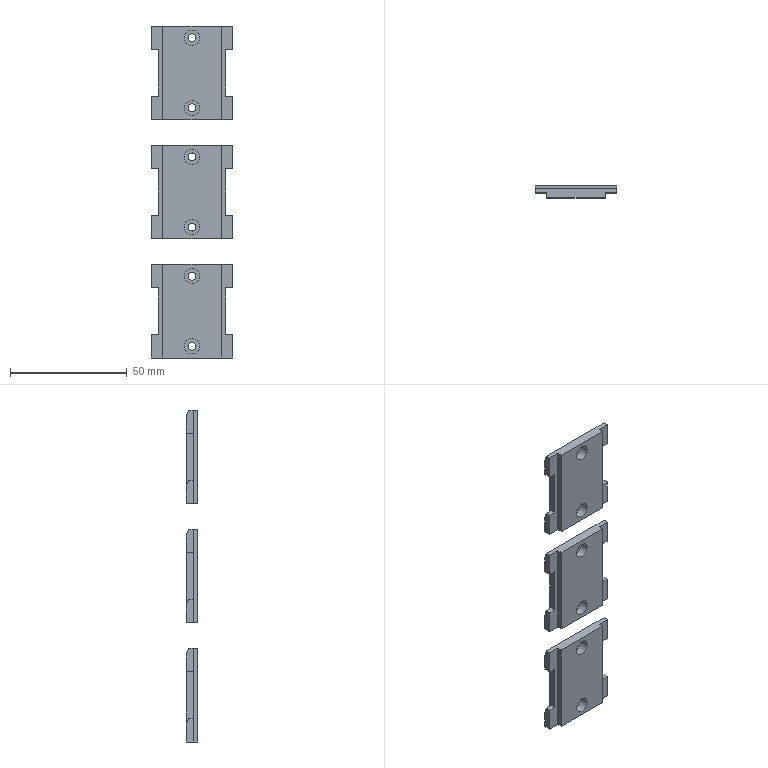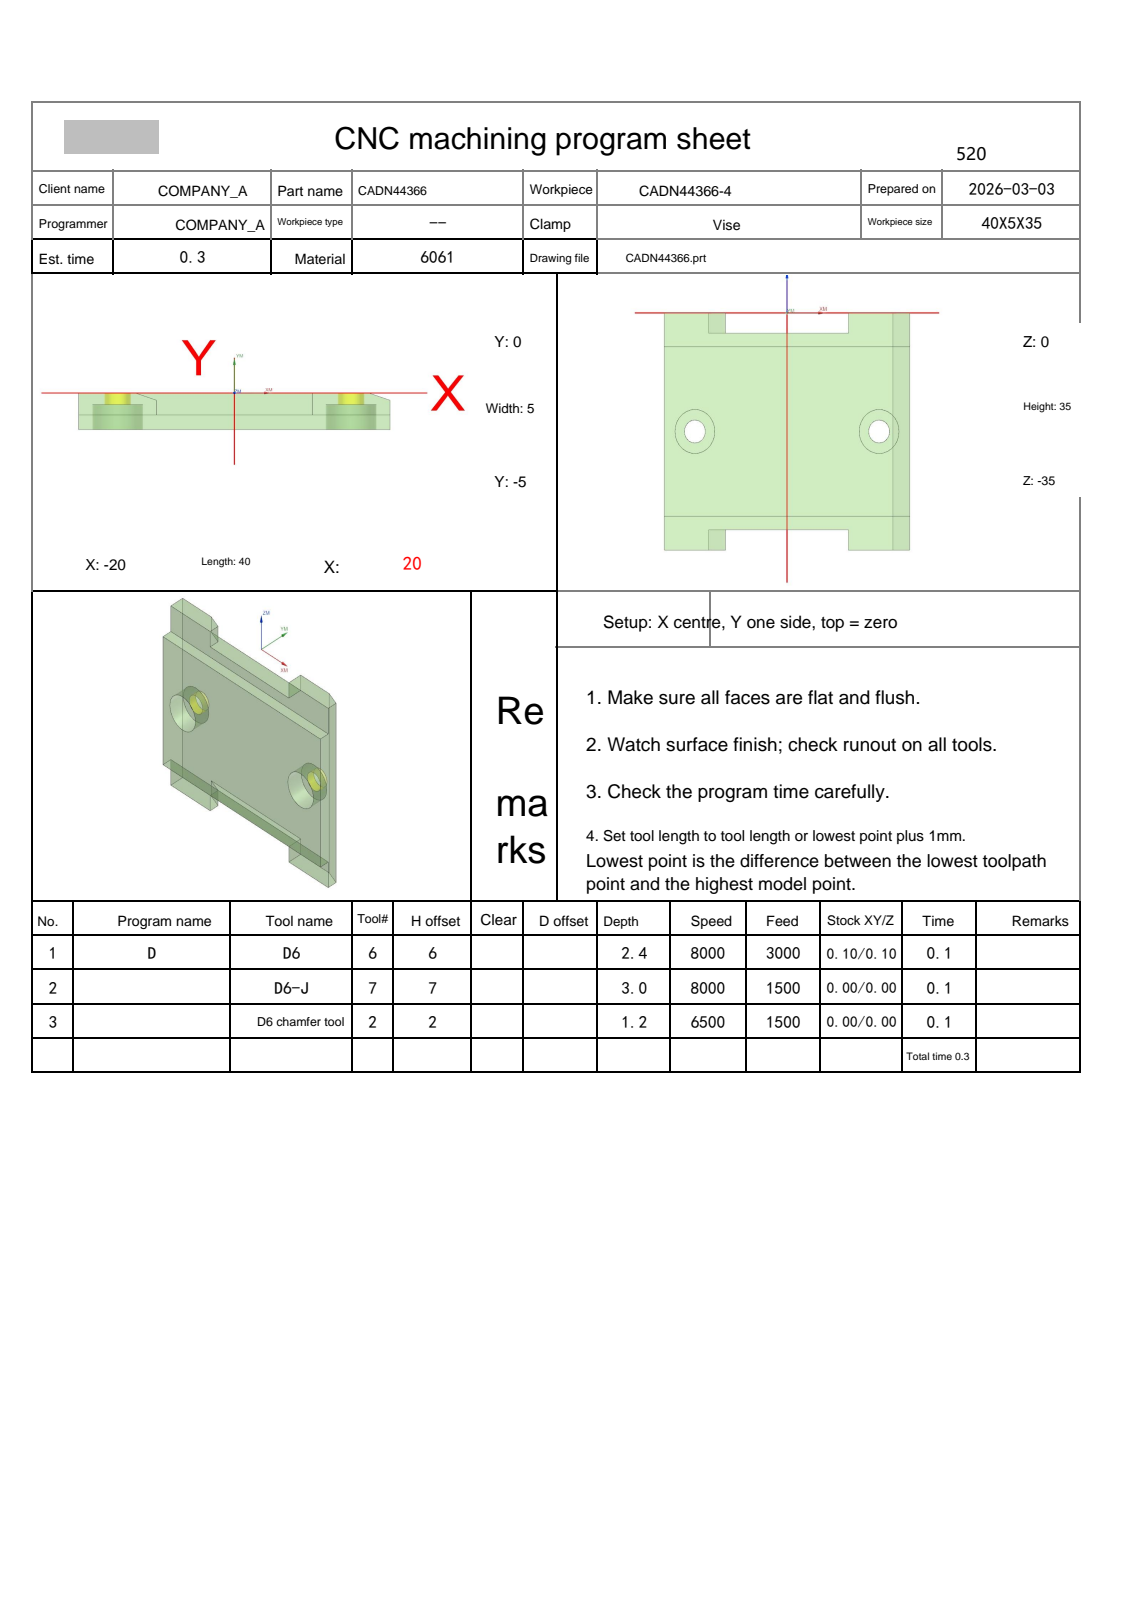NC program | NX | posted by the shop | part box 35 x 5 x 142 mm
Whole program:
%
O0001
(Machine time: 0.80 MIN)
(===Total Tool:3===)
(T6=D6      D=6.   R=0.   D-  H06 Z=-2.4  )
(T7=D6-J    D=6.   R=0.   D7  H07 Z=-3.   )
(T2=D6 chamfer tool   D=6.   R=0.   D-  H02 Z=-1.2  )
G80 G90 G17 G49 G40
G91 G28 Z0
M01
N1 T06 M06
(D6  D=6. R=0. H=06 ce=0.10 di=0.10)
G00 G90 G54 X6.9 Y-8.254 M03 S8000
G43 H06 Z50.
M08
Z-.6
G01 Y-3. F3000.
Y0.0
Y5.254
G00 Z-1.2
G01 Y0.0
Y-3.
Y-8.254
G00 Z-1.8
G01 Y-3.
Y0.0
Y5.254
G00 Z-2.4
G01 Y0.0
Y-3.
Y-8.254
G00 Z50.
X-20.406 Y6.086
Z-.6
G01 X-11.687 Y2.913
X-8.94 Y1.913
G02 X-6.9 Y-1. I-1.06 J-2.913
G01 Y-3.
Y-8.254
G00 Z-1.2
G01 Y-3.
Y-1.
G03 X-8.94 Y1.913 I-3.1 J0.0
G01 X-11.687 Y2.913
X-20.406 Y6.086
G00 Z-1.8
G01 X-11.687 Y2.913
X-8.94 Y1.913
G02 X-6.9 Y-1. I-1.06 J-2.913
G01 Y-3.
Y-8.254
G00 Z-2.4
G01 Y-3.
Y-1.
G03 X-8.94 Y1.913 I-3.1 J0.0
G01 X-11.687 Y2.913
X-20.406 Y6.086
G00 Z50.
G91 G28 Z0.0
M05
M09
G91 G28 Z0.0
M01
N2 T07 M06
(D6-J  D=6. R=0. H=07 ce=0.40 di=0.00)
G00 G90 G54 X1.2 Y-7.2 M03 S7000
G43 H07 Z12.5
M08
Z-1.5
G01 Z-3. F1500.
Y-4.8
G03 X0.0 Y-3.6 I-1.2 J0.0
G01 X-6.001
G02 X-6.6 Y-3.001 I.001 J.6
G01 Y.001
G02 X-6.001 Y.6 I.6 J-.001
G01 X6.001
G02 X6.6 Y.001 I-.001 J-.6
G01 Y-3.001
G02 X6.001 Y-3.6 I-.6 J.001
G01 X0.0
X-1.
G03 X-2.2 Y-4.8 I0.0 J-1.2
G01 Y-7.2
Z-1.5
G00 Z12.5
G00 G90 X-12.985 Y4.4 M03 S8000
Z12.5
Z-2.
G01 Z-3. F1000.
G41 D07
X-12.997 Y4.2
X-13. Y4.125
G03 X-12.21 Y2.997 I1.2 J0.0
G01 X-7. Y1.101
Y-6.
G03 X-5.8 Y-7.2 I1.2 J0.0
G01 G40 X-5.6
Z-2.
G00 X5.6
G01 Z-3.
G41 D07
X5.8
G03 X7. Y-6. I0.0 J1.2
G01 Y3.
G03 X5.8 Y4.2 I-1.2 J0.0
G01 G40 X5.6
Z-2.
G00 Z12.5
G91 G28 Z0.0
M05
M09
G91 G28 Z0.0
M01
N3 T02 M06
(D6 chamfer tool  D=6. R=0. H=02 ce=0.00 di=0.00)
G00 G90 G54 X-14.614 Y-4.227 M03 S6500
G43 H02 Z50.
M08
Z.172
G01 Z-1.2 F1500.
G03 X-14.9 Y-4.027 I-1.286 J-1.532
G01 X-14.946 Y-3.997
X-15. Y-4.
X-20.
G02 X-21. Y-3. I0.0 J1.
G01 Y0.0
G02 X-20. Y1. I1. J0.0
G01 X-12.747
X-12.574 Y.985
X-12.405 Y.94
X-9.658 Y-.06
G02 X-9. Y-1. I-.342 J-.94
G01 Y-3.
G02 X-10. Y-4. I-1. J0.0
G01 X-15.
X-15.054 Y-3.997
X-15.1 Y-4.027
G03 X-15.386 Y-4.227 I1. J-1.732
G01 Z.172
G00 Z10.
X15.386
Z.172
G01 Z-1.2
G03 X15.1 Y-4.027 I-1.286 J-1.532
G01 X15.054 Y-3.997
X15. Y-4.
X10.
G02 X9. Y-3. I0.0 J1.
G01 Y0.0
G02 X10. Y1. I1. J0.0
G01 X17.253
X17.426 Y.985
X17.595 Y.94
X20.342 Y-.06
G02 X21. Y-1. I-.342 J-.94
G01 Y-3.
G02 X20. Y-4. I-1. J0.0
G01 X15.
X14.946 Y-3.997
X14.9 Y-4.027
G03 X14.614 Y-4.227 I1. J-1.732
G01 Z.172
G00 Z50.
M05
M09
G91 G28 Z0.0
G91 G28 Y0.0
M30
%